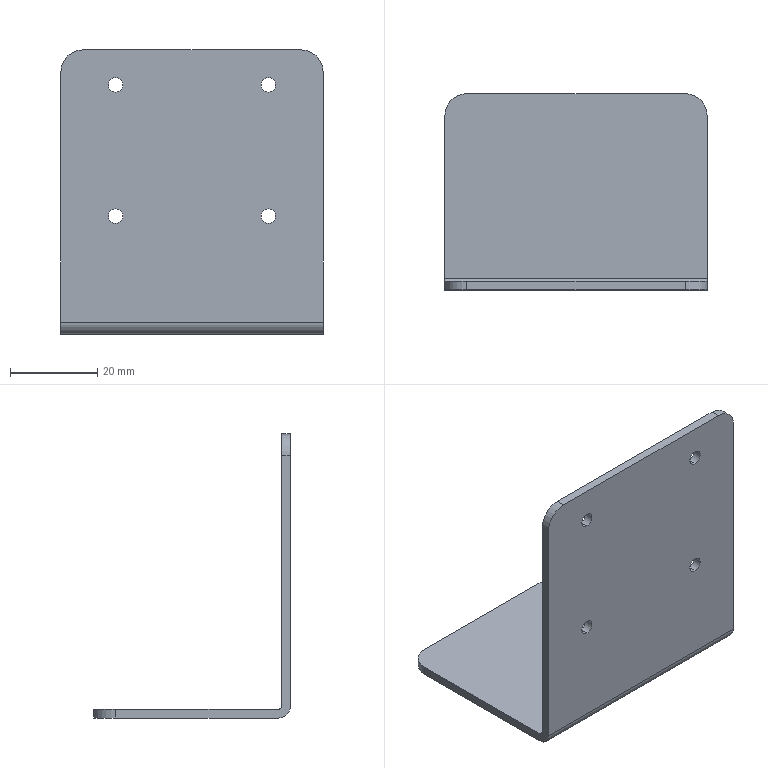Part | 1 solid | 22 faces | box 60 x 45 x 65 mm | volume 12759 mm3 | cylinder 14 | plane 8 | commonest cylinder face diameters 3.3 x8 10 x4 1.48 x1 5.48 x1
STEP:
#1=CARTESIAN_POINT('',(47.5,-2.,-9.65));
#2=VERTEX_POINT('',#1);
#3=CARTESIAN_POINT('',(47.5,-2.,-6.35));
#4=VERTEX_POINT('',#3);
#5=CARTESIAN_POINT('',(47.5,-2.,-8.));
#6=DIRECTION('',(0.,1.,0.));
#7=DIRECTION('',(0.,0.,1.));
#8=AXIS2_PLACEMENT_3D('',#5,#6,#7);
#9=CIRCLE('',#8,1.65);
#10=EDGE_CURVE('',#2,#4,#9,.T.);
#11=ORIENTED_EDGE('',*,*,#10,.F.);
#12=CARTESIAN_POINT('',(47.5,0.,-9.65));
#13=VERTEX_POINT('',#12);
#14=CARTESIAN_POINT('',(47.5,0.,-9.65));
#15=DIRECTION('',(0.,1.,0.));
#16=VECTOR('',#15,1000.);
#17=LINE('',#14,#16);
#18=EDGE_CURVE('',#2,#13,#17,.T.);
#19=ORIENTED_EDGE('',*,*,#18,.T.);
#20=CARTESIAN_POINT('',(47.5,0.,-6.35));
#21=VERTEX_POINT('',#20);
#22=CARTESIAN_POINT('',(47.5,0.,-8.));
#23=DIRECTION('',(0.,1.,0.));
#24=DIRECTION('',(0.,0.,1.));
#25=AXIS2_PLACEMENT_3D('',#22,#23,#24);
#26=CIRCLE('',#25,1.65);
#27=EDGE_CURVE('',#13,#21,#26,.T.);
#28=ORIENTED_EDGE('',*,*,#27,.T.);
#29=CARTESIAN_POINT('',(47.5,0.,-6.35));
#30=DIRECTION('',(0.,1.,0.));
#31=VECTOR('',#30,1000.);
#32=LINE('',#29,#31);
#33=EDGE_CURVE('',#4,#21,#32,.T.);
#34=ORIENTED_EDGE('',*,*,#33,.F.);
#35=EDGE_LOOP('',(#11,#19,#28,#34));
#36=FACE_OUTER_BOUND('',#35,.T.);
#37=CARTESIAN_POINT('',(47.5,0.,-8.));
#38=DIRECTION('',(0.,1.,0.));
#39=DIRECTION('',(0.,0.,1.));
#40=AXIS2_PLACEMENT_3D('',#37,#38,#39);
#41=CYLINDRICAL_SURFACE('',#40,1.65);
#42=ADVANCED_FACE('',(#36),#41,.F.);
#43=CARTESIAN_POINT('',(47.5,-2.,-39.65));
#44=VERTEX_POINT('',#43);
#45=CARTESIAN_POINT('',(47.5,-2.,-36.35));
#46=VERTEX_POINT('',#45);
#47=CARTESIAN_POINT('',(47.5,-2.,-38.));
#48=DIRECTION('',(0.,1.,0.));
#49=DIRECTION('',(0.,0.,1.));
#50=AXIS2_PLACEMENT_3D('',#47,#48,#49);
#51=CIRCLE('',#50,1.65);
#52=EDGE_CURVE('',#44,#46,#51,.T.);
#53=ORIENTED_EDGE('',*,*,#52,.F.);
#54=CARTESIAN_POINT('',(47.5,0.,-39.65));
#55=VERTEX_POINT('',#54);
#56=CARTESIAN_POINT('',(47.5,0.,-39.65));
#57=DIRECTION('',(0.,1.,0.));
#58=VECTOR('',#57,1000.);
#59=LINE('',#56,#58);
#60=EDGE_CURVE('',#44,#55,#59,.T.);
#61=ORIENTED_EDGE('',*,*,#60,.T.);
#62=CARTESIAN_POINT('',(47.5,0.,-36.35));
#63=VERTEX_POINT('',#62);
#64=CARTESIAN_POINT('',(47.5,0.,-38.));
#65=DIRECTION('',(0.,1.,0.));
#66=DIRECTION('',(0.,0.,1.));
#67=AXIS2_PLACEMENT_3D('',#64,#65,#66);
#68=CIRCLE('',#67,1.65);
#69=EDGE_CURVE('',#55,#63,#68,.T.);
#70=ORIENTED_EDGE('',*,*,#69,.T.);
#71=CARTESIAN_POINT('',(47.5,0.,-36.35));
#72=DIRECTION('',(0.,1.,0.));
#73=VECTOR('',#72,1000.);
#74=LINE('',#71,#73);
#75=EDGE_CURVE('',#46,#63,#74,.T.);
#76=ORIENTED_EDGE('',*,*,#75,.F.);
#77=EDGE_LOOP('',(#53,#61,#70,#76));
#78=FACE_OUTER_BOUND('',#77,.T.);
#79=CARTESIAN_POINT('',(47.5,0.,-38.));
#80=DIRECTION('',(0.,1.,0.));
#81=DIRECTION('',(0.,0.,1.));
#82=AXIS2_PLACEMENT_3D('',#79,#80,#81);
#83=CYLINDRICAL_SURFACE('',#82,1.65);
#84=ADVANCED_FACE('',(#78),#83,.F.);
#85=CARTESIAN_POINT('',(12.5,-2.,-9.65));
#86=VERTEX_POINT('',#85);
#87=CARTESIAN_POINT('',(12.5,-2.,-6.35));
#88=VERTEX_POINT('',#87);
#89=CARTESIAN_POINT('',(12.5,-2.,-8.));
#90=DIRECTION('',(0.,1.,0.));
#91=DIRECTION('',(0.,0.,1.));
#92=AXIS2_PLACEMENT_3D('',#89,#90,#91);
#93=CIRCLE('',#92,1.65);
#94=EDGE_CURVE('',#86,#88,#93,.T.);
#95=ORIENTED_EDGE('',*,*,#94,.F.);
#96=CARTESIAN_POINT('',(12.5,0.,-9.65));
#97=VERTEX_POINT('',#96);
#98=CARTESIAN_POINT('',(12.5,0.,-9.65));
#99=DIRECTION('',(0.,1.,0.));
#100=VECTOR('',#99,1000.);
#101=LINE('',#98,#100);
#102=EDGE_CURVE('',#86,#97,#101,.T.);
#103=ORIENTED_EDGE('',*,*,#102,.T.);
#104=CARTESIAN_POINT('',(12.5,0.,-6.35));
#105=VERTEX_POINT('',#104);
#106=CARTESIAN_POINT('',(12.5,0.,-8.));
#107=DIRECTION('',(0.,1.,0.));
#108=DIRECTION('',(0.,0.,1.));
#109=AXIS2_PLACEMENT_3D('',#106,#107,#108);
#110=CIRCLE('',#109,1.65);
#111=EDGE_CURVE('',#97,#105,#110,.T.);
#112=ORIENTED_EDGE('',*,*,#111,.T.);
#113=CARTESIAN_POINT('',(12.5,0.,-6.35));
#114=DIRECTION('',(0.,1.,0.));
#115=VECTOR('',#114,1000.);
#116=LINE('',#113,#115);
#117=EDGE_CURVE('',#88,#105,#116,.T.);
#118=ORIENTED_EDGE('',*,*,#117,.F.);
#119=EDGE_LOOP('',(#95,#103,#112,#118));
#120=FACE_OUTER_BOUND('',#119,.T.);
#121=CARTESIAN_POINT('',(12.5,0.,-8.));
#122=DIRECTION('',(0.,1.,0.));
#123=DIRECTION('',(0.,0.,1.));
#124=AXIS2_PLACEMENT_3D('',#121,#122,#123);
#125=CYLINDRICAL_SURFACE('',#124,1.65);
#126=ADVANCED_FACE('',(#120),#125,.F.);
#127=CARTESIAN_POINT('',(12.5,-2.,-39.65));
#128=VERTEX_POINT('',#127);
#129=CARTESIAN_POINT('',(12.5,-2.,-36.35));
#130=VERTEX_POINT('',#129);
#131=CARTESIAN_POINT('',(12.5,-2.,-38.));
#132=DIRECTION('',(0.,1.,0.));
#133=DIRECTION('',(0.,0.,1.));
#134=AXIS2_PLACEMENT_3D('',#131,#132,#133);
#135=CIRCLE('',#134,1.65);
#136=EDGE_CURVE('',#128,#130,#135,.T.);
#137=ORIENTED_EDGE('',*,*,#136,.F.);
#138=CARTESIAN_POINT('',(12.5,0.,-39.65));
#139=VERTEX_POINT('',#138);
#140=CARTESIAN_POINT('',(12.5,0.,-39.65));
#141=DIRECTION('',(0.,1.,0.));
#142=VECTOR('',#141,1000.);
#143=LINE('',#140,#142);
#144=EDGE_CURVE('',#128,#139,#143,.T.);
#145=ORIENTED_EDGE('',*,*,#144,.T.);
#146=CARTESIAN_POINT('',(12.5,0.,-36.35));
#147=VERTEX_POINT('',#146);
#148=CARTESIAN_POINT('',(12.5,0.,-38.));
#149=DIRECTION('',(0.,1.,0.));
#150=DIRECTION('',(0.,0.,1.));
#151=AXIS2_PLACEMENT_3D('',#148,#149,#150);
#152=CIRCLE('',#151,1.65);
#153=EDGE_CURVE('',#139,#147,#152,.T.);
#154=ORIENTED_EDGE('',*,*,#153,.T.);
#155=CARTESIAN_POINT('',(12.5,0.,-36.35));
#156=DIRECTION('',(0.,1.,0.));
#157=VECTOR('',#156,1000.);
#158=LINE('',#155,#157);
#159=EDGE_CURVE('',#130,#147,#158,.T.);
#160=ORIENTED_EDGE('',*,*,#159,.F.);
#161=EDGE_LOOP('',(#137,#145,#154,#160));
#162=FACE_OUTER_BOUND('',#161,.T.);
#163=CARTESIAN_POINT('',(12.5,0.,-38.));
#164=DIRECTION('',(0.,1.,0.));
#165=DIRECTION('',(0.,0.,1.));
#166=AXIS2_PLACEMENT_3D('',#163,#164,#165);
#167=CYLINDRICAL_SURFACE('',#166,1.65);
#168=ADVANCED_FACE('',(#162),#167,.F.);
#169=CARTESIAN_POINT('',(0.,-2.,-62.26));
#170=VERTEX_POINT('',#169);
#171=CARTESIAN_POINT('',(0.,-2.,-5.));
#172=VERTEX_POINT('',#171);
#173=CARTESIAN_POINT('',(0.,-2.,0.));
#174=DIRECTION('',(0.,0.,1.));
#175=VECTOR('',#174,1000.);
#176=LINE('',#173,#175);
#177=EDGE_CURVE('',#170,#172,#176,.T.);
#178=ORIENTED_EDGE('',*,*,#177,.T.);
#179=CARTESIAN_POINT('',(0.,0.,-5.));
#180=VERTEX_POINT('',#179);
#181=CARTESIAN_POINT('',(0.,-2.,-5.));
#182=DIRECTION('',(0.,1.,0.));
#183=VECTOR('',#182,1000.);
#184=LINE('',#181,#183);
#185=EDGE_CURVE('',#172,#180,#184,.T.);
#186=ORIENTED_EDGE('',*,*,#185,.T.);
#187=CARTESIAN_POINT('',(0.,0.,-62.26));
#188=VERTEX_POINT('',#187);
#189=CARTESIAN_POINT('',(0.,0.,0.));
#190=DIRECTION('',(0.,0.,1.));
#191=VECTOR('',#190,1000.);
#192=LINE('',#189,#191);
#193=EDGE_CURVE('',#188,#180,#192,.T.);
#194=ORIENTED_EDGE('',*,*,#193,.F.);
#195=CARTESIAN_POINT('',(0.,0.74,-63.));
#196=VERTEX_POINT('',#195);
#197=CARTESIAN_POINT('',(0.,0.74,-62.26));
#198=DIRECTION('',(-1.,0.,0.));
#199=DIRECTION('',(0.,0.,1.));
#200=AXIS2_PLACEMENT_3D('',#197,#198,#199);
#201=CIRCLE('',#200,0.74);
#202=EDGE_CURVE('',#196,#188,#201,.T.);
#203=ORIENTED_EDGE('',*,*,#202,.F.);
#204=CARTESIAN_POINT('',(0.,38.,-63.));
#205=VERTEX_POINT('',#204);
#206=CARTESIAN_POINT('',(0.,0.,-63.));
#207=DIRECTION('',(0.,-1.,0.));
#208=VECTOR('',#207,1000.);
#209=LINE('',#206,#208);
#210=EDGE_CURVE('',#205,#196,#209,.T.);
#211=ORIENTED_EDGE('',*,*,#210,.F.);
#212=CARTESIAN_POINT('',(0.,38.,-65.));
#213=VERTEX_POINT('',#212);
#214=CARTESIAN_POINT('',(0.,38.,-65.));
#215=DIRECTION('',(0.,0.,-1.));
#216=VECTOR('',#215,1000.);
#217=LINE('',#214,#216);
#218=EDGE_CURVE('',#205,#213,#217,.T.);
#219=ORIENTED_EDGE('',*,*,#218,.T.);
#220=CARTESIAN_POINT('',(0.,0.74,-65.));
#221=VERTEX_POINT('',#220);
#222=CARTESIAN_POINT('',(0.,0.,-65.));
#223=DIRECTION('',(0.,-1.,0.));
#224=VECTOR('',#223,1000.);
#225=LINE('',#222,#224);
#226=EDGE_CURVE('',#213,#221,#225,.T.);
#227=ORIENTED_EDGE('',*,*,#226,.T.);
#228=CARTESIAN_POINT('',(0.,0.74,-62.26));
#229=DIRECTION('',(-1.,0.,0.));
#230=DIRECTION('',(0.,0.,1.));
#231=AXIS2_PLACEMENT_3D('',#228,#229,#230);
#232=CIRCLE('',#231,2.74);
#233=EDGE_CURVE('',#221,#170,#232,.T.);
#234=ORIENTED_EDGE('',*,*,#233,.T.);
#235=EDGE_LOOP('',(#178,#186,#194,#203,#211,#219,#227,#234));
#236=FACE_OUTER_BOUND('',#235,.T.);
#237=CARTESIAN_POINT('',(0.,-2.,0.));
#238=DIRECTION('',(-1.,0.,0.));
#239=DIRECTION('',(0.,0.,1.));
#240=AXIS2_PLACEMENT_3D('',#237,#238,#239);
#241=PLANE('',#240);
#242=ADVANCED_FACE('',(#236),#241,.T.);
#243=CARTESIAN_POINT('',(47.5,-2.,-8.));
#244=DIRECTION('',(0.,1.,0.));
#245=DIRECTION('',(0.,0.,1.));
#246=AXIS2_PLACEMENT_3D('',#243,#244,#245);
#247=CIRCLE('',#246,1.65);
#248=EDGE_CURVE('',#4,#2,#247,.T.);
#249=ORIENTED_EDGE('',*,*,#248,.T.);
#250=ORIENTED_EDGE('',*,*,#10,.T.);
#251=EDGE_LOOP('',(#249,#250));
#252=FACE_BOUND('',#251,.T.);
#253=CARTESIAN_POINT('',(47.5,-2.,-38.));
#254=DIRECTION('',(0.,1.,0.));
#255=DIRECTION('',(0.,0.,1.));
#256=AXIS2_PLACEMENT_3D('',#253,#254,#255);
#257=CIRCLE('',#256,1.65);
#258=EDGE_CURVE('',#46,#44,#257,.T.);
#259=ORIENTED_EDGE('',*,*,#258,.T.);
#260=ORIENTED_EDGE('',*,*,#52,.T.);
#261=EDGE_LOOP('',(#259,#260));
#262=FACE_BOUND('',#261,.T.);
#263=CARTESIAN_POINT('',(12.5,-2.,-8.));
#264=DIRECTION('',(0.,1.,0.));
#265=DIRECTION('',(0.,0.,1.));
#266=AXIS2_PLACEMENT_3D('',#263,#264,#265);
#267=CIRCLE('',#266,1.65);
#268=EDGE_CURVE('',#88,#86,#267,.T.);
#269=ORIENTED_EDGE('',*,*,#268,.T.);
#270=ORIENTED_EDGE('',*,*,#94,.T.);
#271=EDGE_LOOP('',(#269,#270));
#272=FACE_BOUND('',#271,.T.);
#273=CARTESIAN_POINT('',(12.5,-2.,-38.));
#274=DIRECTION('',(0.,1.,0.));
#275=DIRECTION('',(0.,0.,1.));
#276=AXIS2_PLACEMENT_3D('',#273,#274,#275);
#277=CIRCLE('',#276,1.65);
#278=EDGE_CURVE('',#130,#128,#277,.T.);
#279=ORIENTED_EDGE('',*,*,#278,.T.);
#280=ORIENTED_EDGE('',*,*,#136,.T.);
#281=EDGE_LOOP('',(#279,#280));
#282=FACE_BOUND('',#281,.T.);
#283=CARTESIAN_POINT('',(60.,-2.,-5.));
#284=VERTEX_POINT('',#283);
#285=CARTESIAN_POINT('',(60.,-2.,-62.26));
#286=VERTEX_POINT('',#285);
#287=CARTESIAN_POINT('',(60.,-2.,0.));
#288=DIRECTION('',(0.,0.,-1.));
#289=VECTOR('',#288,1000.);
#290=LINE('',#287,#289);
#291=EDGE_CURVE('',#284,#286,#290,.T.);
#292=ORIENTED_EDGE('',*,*,#291,.F.);
#293=CARTESIAN_POINT('',(55.,-2.,0.));
#294=VERTEX_POINT('',#293);
#295=CARTESIAN_POINT('',(55.,-2.,-5.));
#296=DIRECTION('',(0.,-1.,0.));
#297=DIRECTION('',(0.,0.,-1.));
#298=AXIS2_PLACEMENT_3D('',#295,#296,#297);
#299=CIRCLE('',#298,5.);
#300=EDGE_CURVE('',#284,#294,#299,.T.);
#301=ORIENTED_EDGE('',*,*,#300,.T.);
#302=CARTESIAN_POINT('',(5.,-2.,0.));
#303=VERTEX_POINT('',#302);
#304=CARTESIAN_POINT('',(0.,-2.,0.));
#305=DIRECTION('',(1.,0.,0.));
#306=VECTOR('',#305,1000.);
#307=LINE('',#304,#306);
#308=EDGE_CURVE('',#303,#294,#307,.T.);
#309=ORIENTED_EDGE('',*,*,#308,.F.);
#310=CARTESIAN_POINT('',(5.,-2.,-5.));
#311=DIRECTION('',(0.,-1.,0.));
#312=DIRECTION('',(0.,0.,-1.));
#313=AXIS2_PLACEMENT_3D('',#310,#311,#312);
#314=CIRCLE('',#313,5.);
#315=EDGE_CURVE('',#303,#172,#314,.T.);
#316=ORIENTED_EDGE('',*,*,#315,.T.);
#317=ORIENTED_EDGE('',*,*,#177,.F.);
#318=CARTESIAN_POINT('',(0.,-2.,-62.26));
#319=DIRECTION('',(1.,0.,0.));
#320=VECTOR('',#319,1000.);
#321=LINE('',#318,#320);
#322=EDGE_CURVE('',#170,#286,#321,.T.);
#323=ORIENTED_EDGE('',*,*,#322,.T.);
#324=EDGE_LOOP('',(#292,#301,#309,#316,#317,#323));
#325=FACE_OUTER_BOUND('',#324,.T.);
#326=CARTESIAN_POINT('',(0.,-2.,0.));
#327=DIRECTION('',(0.,-1.,0.));
#328=DIRECTION('',(0.,0.,-1.));
#329=AXIS2_PLACEMENT_3D('',#326,#327,#328);
#330=PLANE('',#329);
#331=ADVANCED_FACE('',(#252,#262,#272,#282,#325),#330,.T.);
#332=CARTESIAN_POINT('',(47.5,0.,-8.));
#333=DIRECTION('',(0.,1.,0.));
#334=DIRECTION('',(0.,0.,1.));
#335=AXIS2_PLACEMENT_3D('',#332,#333,#334);
#336=CIRCLE('',#335,1.65);
#337=EDGE_CURVE('',#21,#13,#336,.T.);
#338=ORIENTED_EDGE('',*,*,#337,.F.);
#339=ORIENTED_EDGE('',*,*,#27,.F.);
#340=EDGE_LOOP('',(#338,#339));
#341=FACE_BOUND('',#340,.T.);
#342=CARTESIAN_POINT('',(47.5,0.,-38.));
#343=DIRECTION('',(0.,1.,0.));
#344=DIRECTION('',(0.,0.,1.));
#345=AXIS2_PLACEMENT_3D('',#342,#343,#344);
#346=CIRCLE('',#345,1.65);
#347=EDGE_CURVE('',#63,#55,#346,.T.);
#348=ORIENTED_EDGE('',*,*,#347,.F.);
#349=ORIENTED_EDGE('',*,*,#69,.F.);
#350=EDGE_LOOP('',(#348,#349));
#351=FACE_BOUND('',#350,.T.);
#352=CARTESIAN_POINT('',(12.5,0.,-8.));
#353=DIRECTION('',(0.,1.,0.));
#354=DIRECTION('',(0.,0.,1.));
#355=AXIS2_PLACEMENT_3D('',#352,#353,#354);
#356=CIRCLE('',#355,1.65);
#357=EDGE_CURVE('',#105,#97,#356,.T.);
#358=ORIENTED_EDGE('',*,*,#357,.F.);
#359=ORIENTED_EDGE('',*,*,#111,.F.);
#360=EDGE_LOOP('',(#358,#359));
#361=FACE_BOUND('',#360,.T.);
#362=CARTESIAN_POINT('',(12.5,0.,-38.));
#363=DIRECTION('',(0.,1.,0.));
#364=DIRECTION('',(0.,0.,1.));
#365=AXIS2_PLACEMENT_3D('',#362,#363,#364);
#366=CIRCLE('',#365,1.65);
#367=EDGE_CURVE('',#147,#139,#366,.T.);
#368=ORIENTED_EDGE('',*,*,#367,.F.);
#369=ORIENTED_EDGE('',*,*,#153,.F.);
#370=EDGE_LOOP('',(#368,#369));
#371=FACE_BOUND('',#370,.T.);
#372=CARTESIAN_POINT('',(5.,0.,0.));
#373=VERTEX_POINT('',#372);
#374=CARTESIAN_POINT('',(55.,0.,0.));
#375=VERTEX_POINT('',#374);
#376=CARTESIAN_POINT('',(0.,0.,0.));
#377=DIRECTION('',(1.,0.,0.));
#378=VECTOR('',#377,1000.);
#379=LINE('',#376,#378);
#380=EDGE_CURVE('',#373,#375,#379,.T.);
#381=ORIENTED_EDGE('',*,*,#380,.T.);
#382=CARTESIAN_POINT('',(60.,0.,-5.));
#383=VERTEX_POINT('',#382);
#384=CARTESIAN_POINT('',(55.,0.,-5.));
#385=DIRECTION('',(0.,1.,0.));
#386=DIRECTION('',(0.,0.,-1.));
#387=AXIS2_PLACEMENT_3D('',#384,#385,#386);
#388=CIRCLE('',#387,5.);
#389=EDGE_CURVE('',#375,#383,#388,.T.);
#390=ORIENTED_EDGE('',*,*,#389,.T.);
#391=CARTESIAN_POINT('',(60.,0.,-62.26));
#392=VERTEX_POINT('',#391);
#393=CARTESIAN_POINT('',(60.,0.,0.));
#394=DIRECTION('',(0.,0.,-1.));
#395=VECTOR('',#394,1000.);
#396=LINE('',#393,#395);
#397=EDGE_CURVE('',#383,#392,#396,.T.);
#398=ORIENTED_EDGE('',*,*,#397,.T.);
#399=CARTESIAN_POINT('',(0.,0.,-62.26));
#400=DIRECTION('',(1.,0.,0.));
#401=VECTOR('',#400,1000.);
#402=LINE('',#399,#401);
#403=EDGE_CURVE('',#188,#392,#402,.T.);
#404=ORIENTED_EDGE('',*,*,#403,.F.);
#405=ORIENTED_EDGE('',*,*,#193,.T.);
#406=CARTESIAN_POINT('',(5.,0.,-5.));
#407=DIRECTION('',(0.,1.,0.));
#408=DIRECTION('',(0.,0.,-1.));
#409=AXIS2_PLACEMENT_3D('',#406,#407,#408);
#410=CIRCLE('',#409,5.);
#411=EDGE_CURVE('',#180,#373,#410,.T.);
#412=ORIENTED_EDGE('',*,*,#411,.T.);
#413=EDGE_LOOP('',(#381,#390,#398,#404,#405,#412));
#414=FACE_OUTER_BOUND('',#413,.T.);
#415=CARTESIAN_POINT('',(0.,0.,0.));
#416=DIRECTION('',(0.,-1.,0.));
#417=DIRECTION('',(0.,0.,-1.));
#418=AXIS2_PLACEMENT_3D('',#415,#416,#417);
#419=PLANE('',#418);
#420=ADVANCED_FACE('',(#341,#351,#361,#371,#414),#419,.F.);
#421=ORIENTED_EDGE('',*,*,#397,.F.);
#422=CARTESIAN_POINT('',(60.,-2.,-5.));
#423=DIRECTION('',(0.,-1.,0.));
#424=VECTOR('',#423,1000.);
#425=LINE('',#422,#424);
#426=EDGE_CURVE('',#383,#284,#425,.T.);
#427=ORIENTED_EDGE('',*,*,#426,.T.);
#428=ORIENTED_EDGE('',*,*,#291,.T.);
#429=CARTESIAN_POINT('',(60.,0.74,-65.));
#430=VERTEX_POINT('',#429);
#431=CARTESIAN_POINT('',(60.,0.74,-62.26));
#432=DIRECTION('',(1.,0.,0.));
#433=DIRECTION('',(0.,0.,1.));
#434=AXIS2_PLACEMENT_3D('',#431,#432,#433);
#435=CIRCLE('',#434,2.74);
#436=EDGE_CURVE('',#286,#430,#435,.T.);
#437=ORIENTED_EDGE('',*,*,#436,.T.);
#438=CARTESIAN_POINT('',(60.,38.,-65.));
#439=VERTEX_POINT('',#438);
#440=CARTESIAN_POINT('',(60.,43.,-65.));
#441=DIRECTION('',(0.,1.,0.));
#442=VECTOR('',#441,1000.);
#443=LINE('',#440,#442);
#444=EDGE_CURVE('',#430,#439,#443,.T.);
#445=ORIENTED_EDGE('',*,*,#444,.T.);
#446=CARTESIAN_POINT('',(60.,38.,-63.));
#447=VERTEX_POINT('',#446);
#448=CARTESIAN_POINT('',(60.,38.,-65.));
#449=DIRECTION('',(0.,0.,1.));
#450=VECTOR('',#449,1000.);
#451=LINE('',#448,#450);
#452=EDGE_CURVE('',#439,#447,#451,.T.);
#453=ORIENTED_EDGE('',*,*,#452,.T.);
#454=CARTESIAN_POINT('',(60.,0.74,-63.));
#455=VERTEX_POINT('',#454);
#456=CARTESIAN_POINT('',(60.,0.,-63.));
#457=DIRECTION('',(0.,1.,0.));
#458=VECTOR('',#457,1000.);
#459=LINE('',#456,#458);
#460=EDGE_CURVE('',#455,#447,#459,.T.);
#461=ORIENTED_EDGE('',*,*,#460,.F.);
#462=CARTESIAN_POINT('',(60.,0.74,-62.26));
#463=DIRECTION('',(1.,0.,0.));
#464=DIRECTION('',(0.,0.,1.));
#465=AXIS2_PLACEMENT_3D('',#462,#463,#464);
#466=CIRCLE('',#465,0.74);
#467=EDGE_CURVE('',#392,#455,#466,.T.);
#468=ORIENTED_EDGE('',*,*,#467,.F.);
#469=EDGE_LOOP('',(#421,#427,#428,#437,#445,#453,#461,#468));
#470=FACE_OUTER_BOUND('',#469,.T.);
#471=CARTESIAN_POINT('',(60.,-2.,0.));
#472=DIRECTION('',(1.,0.,0.));
#473=DIRECTION('',(0.,0.,-1.));
#474=AXIS2_PLACEMENT_3D('',#471,#472,#473);
#475=PLANE('',#474);
#476=ADVANCED_FACE('',(#470),#475,.T.);
#477=ORIENTED_EDGE('',*,*,#308,.T.);
#478=CARTESIAN_POINT('',(55.,-2.,0.));
#479=DIRECTION('',(0.,1.,0.));
#480=VECTOR('',#479,1000.);
#481=LINE('',#478,#480);
#482=EDGE_CURVE('',#294,#375,#481,.T.);
#483=ORIENTED_EDGE('',*,*,#482,.T.);
#484=ORIENTED_EDGE('',*,*,#380,.F.);
#485=CARTESIAN_POINT('',(5.,-2.,0.));
#486=DIRECTION('',(0.,-1.,0.));
#487=VECTOR('',#486,1000.);
#488=LINE('',#485,#487);
#489=EDGE_CURVE('',#373,#303,#488,.T.);
#490=ORIENTED_EDGE('',*,*,#489,.T.);
#491=EDGE_LOOP('',(#477,#483,#484,#490));
#492=FACE_OUTER_BOUND('',#491,.T.);
#493=CARTESIAN_POINT('',(0.,-2.,0.));
#494=DIRECTION('',(0.,0.,1.));
#495=DIRECTION('',(1.,0.,0.));
#496=AXIS2_PLACEMENT_3D('',#493,#494,#495);
#497=PLANE('',#496);
#498=ADVANCED_FACE('',(#492),#497,.T.);
#499=ORIENTED_EDGE('',*,*,#322,.F.);
#500=ORIENTED_EDGE('',*,*,#233,.F.);
#501=CARTESIAN_POINT('',(0.,0.74,-65.));
#502=DIRECTION('',(-1.,0.,0.));
#503=VECTOR('',#502,1000.);
#504=LINE('',#501,#503);
#505=EDGE_CURVE('',#430,#221,#504,.T.);
#506=ORIENTED_EDGE('',*,*,#505,.F.);
#507=ORIENTED_EDGE('',*,*,#436,.F.);
#508=EDGE_LOOP('',(#499,#500,#506,#507));
#509=FACE_OUTER_BOUND('',#508,.T.);
#510=CARTESIAN_POINT('',(0.,0.74,-62.26));
#511=DIRECTION('',(-1.,0.,0.));
#512=DIRECTION('',(0.,0.,-1.));
#513=AXIS2_PLACEMENT_3D('',#510,#511,#512);
#514=CYLINDRICAL_SURFACE('',#513,2.74);
#515=ADVANCED_FACE('',(#509),#514,.T.);
#516=ORIENTED_EDGE('',*,*,#403,.T.);
#517=ORIENTED_EDGE('',*,*,#467,.T.);
#518=CARTESIAN_POINT('',(60.,0.74,-63.));
#519=DIRECTION('',(-1.,0.,0.));
#520=VECTOR('',#519,1000.);
#521=LINE('',#518,#520);
#522=EDGE_CURVE('',#455,#196,#521,.T.);
#523=ORIENTED_EDGE('',*,*,#522,.T.);
#524=ORIENTED_EDGE('',*,*,#202,.T.);
#525=EDGE_LOOP('',(#516,#517,#523,#524));
#526=FACE_OUTER_BOUND('',#525,.T.);
#527=CARTESIAN_POINT('',(0.,0.74,-62.26));
#528=DIRECTION('',(-1.,0.,0.));
#529=DIRECTION('',(0.,0.,-1.));
#530=AXIS2_PLACEMENT_3D('',#527,#528,#529);
#531=CYLINDRICAL_SURFACE('',#530,0.74);
#532=ADVANCED_FACE('',(#526),#531,.F.);
#533=ORIENTED_EDGE('',*,*,#226,.F.);
#534=CARTESIAN_POINT('',(5.,43.,-65.));
#535=VERTEX_POINT('',#534);
#536=CARTESIAN_POINT('',(5.,38.,-65.));
#537=DIRECTION('',(0.,0.,-1.));
#538=DIRECTION('',(-1.,0.,0.));
#539=AXIS2_PLACEMENT_3D('',#536,#537,#538);
#540=CIRCLE('',#539,5.);
#541=EDGE_CURVE('',#213,#535,#540,.T.);
#542=ORIENTED_EDGE('',*,*,#541,.T.);
#543=CARTESIAN_POINT('',(55.,43.,-65.));
#544=VERTEX_POINT('',#543);
#545=CARTESIAN_POINT('',(0.,43.,-65.));
#546=DIRECTION('',(-1.,0.,0.));
#547=VECTOR('',#546,1000.);
#548=LINE('',#545,#547);
#549=EDGE_CURVE('',#544,#535,#548,.T.);
#550=ORIENTED_EDGE('',*,*,#549,.F.);
#551=CARTESIAN_POINT('',(55.,38.,-65.));
#552=DIRECTION('',(0.,0.,-1.));
#553=DIRECTION('',(-1.,0.,0.));
#554=AXIS2_PLACEMENT_3D('',#551,#552,#553);
#555=CIRCLE('',#554,5.);
#556=EDGE_CURVE('',#544,#439,#555,.T.);
#557=ORIENTED_EDGE('',*,*,#556,.T.);
#558=ORIENTED_EDGE('',*,*,#444,.F.);
#559=ORIENTED_EDGE('',*,*,#505,.T.);
#560=EDGE_LOOP('',(#533,#542,#550,#557,#558,#559));
#561=FACE_OUTER_BOUND('',#560,.T.);
#562=CARTESIAN_POINT('',(0.,0.,-65.));
#563=DIRECTION('',(0.,0.,-1.));
#564=DIRECTION('',(-1.,0.,0.));
#565=AXIS2_PLACEMENT_3D('',#562,#563,#564);
#566=PLANE('',#565);
#567=ADVANCED_FACE('',(#561),#566,.T.);
#568=CARTESIAN_POINT('',(55.,43.,-63.));
#569=VERTEX_POINT('',#568);
#570=CARTESIAN_POINT('',(5.,43.,-63.));
#571=VERTEX_POINT('',#570);
#572=CARTESIAN_POINT('',(0.,43.,-63.));
#573=DIRECTION('',(-1.,0.,0.));
#574=VECTOR('',#573,1000.);
#575=LINE('',#572,#574);
#576=EDGE_CURVE('',#569,#571,#575,.T.);
#577=ORIENTED_EDGE('',*,*,#576,.T.);
#578=CARTESIAN_POINT('',(5.,38.,-63.));
#579=DIRECTION('',(0.,0.,1.));
#580=DIRECTION('',(-1.,0.,0.));
#581=AXIS2_PLACEMENT_3D('',#578,#579,#580);
#582=CIRCLE('',#581,5.);
#583=EDGE_CURVE('',#571,#205,#582,.T.);
#584=ORIENTED_EDGE('',*,*,#583,.T.);
#585=ORIENTED_EDGE('',*,*,#210,.T.);
#586=ORIENTED_EDGE('',*,*,#522,.F.);
#587=ORIENTED_EDGE('',*,*,#460,.T.);
#588=CARTESIAN_POINT('',(55.,38.,-63.));
#589=DIRECTION('',(0.,0.,1.));
#590=DIRECTION('',(-1.,0.,0.));
#591=AXIS2_PLACEMENT_3D('',#588,#589,#590);
#592=CIRCLE('',#591,5.);
#593=EDGE_CURVE('',#447,#569,#592,.T.);
#594=ORIENTED_EDGE('',*,*,#593,.T.);
#595=EDGE_LOOP('',(#577,#584,#585,#586,#587,#594));
#596=FACE_OUTER_BOUND('',#595,.T.);
#597=CARTESIAN_POINT('',(0.,0.,-63.));
#598=DIRECTION('',(0.,0.,-1.));
#599=DIRECTION('',(-1.,0.,0.));
#600=AXIS2_PLACEMENT_3D('',#597,#598,#599);
#601=PLANE('',#600);
#602=ADVANCED_FACE('',(#596),#601,.F.);
#603=ORIENTED_EDGE('',*,*,#549,.T.);
#604=CARTESIAN_POINT('',(5.,43.,-65.));
#605=DIRECTION('',(0.,0.,1.));
#606=VECTOR('',#605,1000.);
#607=LINE('',#604,#606);
#608=EDGE_CURVE('',#535,#571,#607,.T.);
#609=ORIENTED_EDGE('',*,*,#608,.T.);
#610=ORIENTED_EDGE('',*,*,#576,.F.);
#611=CARTESIAN_POINT('',(55.,43.,-65.));
#612=DIRECTION('',(0.,0.,-1.));
#613=VECTOR('',#612,1000.);
#614=LINE('',#611,#613);
#615=EDGE_CURVE('',#569,#544,#614,.T.);
#616=ORIENTED_EDGE('',*,*,#615,.T.);
#617=EDGE_LOOP('',(#603,#609,#610,#616));
#618=FACE_OUTER_BOUND('',#617,.T.);
#619=CARTESIAN_POINT('',(0.,43.,-65.));
#620=DIRECTION('',(0.,1.,0.));
#621=DIRECTION('',(0.,0.,1.));
#622=AXIS2_PLACEMENT_3D('',#619,#620,#621);
#623=PLANE('',#622);
#624=ADVANCED_FACE('',(#618),#623,.T.);
#625=ORIENTED_EDGE('',*,*,#541,.F.);
#626=ORIENTED_EDGE('',*,*,#218,.F.);
#627=ORIENTED_EDGE('',*,*,#583,.F.);
#628=ORIENTED_EDGE('',*,*,#608,.F.);
#629=EDGE_LOOP('',(#625,#626,#627,#628));
#630=FACE_OUTER_BOUND('',#629,.T.);
#631=CARTESIAN_POINT('',(5.,38.,-65.));
#632=DIRECTION('',(0.,0.,1.));
#633=DIRECTION('',(1.,0.,0.));
#634=AXIS2_PLACEMENT_3D('',#631,#632,#633);
#635=CYLINDRICAL_SURFACE('',#634,5.);
#636=ADVANCED_FACE('',(#630),#635,.T.);
#637=ORIENTED_EDGE('',*,*,#556,.F.);
#638=ORIENTED_EDGE('',*,*,#615,.F.);
#639=ORIENTED_EDGE('',*,*,#593,.F.);
#640=ORIENTED_EDGE('',*,*,#452,.F.);
#641=EDGE_LOOP('',(#637,#638,#639,#640));
#642=FACE_OUTER_BOUND('',#641,.T.);
#643=CARTESIAN_POINT('',(55.,38.,-65.));
#644=DIRECTION('',(0.,0.,1.));
#645=DIRECTION('',(1.,0.,0.));
#646=AXIS2_PLACEMENT_3D('',#643,#644,#645);
#647=CYLINDRICAL_SURFACE('',#646,5.);
#648=ADVANCED_FACE('',(#642),#647,.T.);
#649=ORIENTED_EDGE('',*,*,#300,.F.);
#650=ORIENTED_EDGE('',*,*,#426,.F.);
#651=ORIENTED_EDGE('',*,*,#389,.F.);
#652=ORIENTED_EDGE('',*,*,#482,.F.);
#653=EDGE_LOOP('',(#649,#650,#651,#652));
#654=FACE_OUTER_BOUND('',#653,.T.);
#655=CARTESIAN_POINT('',(55.,-2.,-5.));
#656=DIRECTION('',(0.,1.,0.));
#657=DIRECTION('',(0.,0.,1.));
#658=AXIS2_PLACEMENT_3D('',#655,#656,#657);
#659=CYLINDRICAL_SURFACE('',#658,5.);
#660=ADVANCED_FACE('',(#654),#659,.T.);
#661=ORIENTED_EDGE('',*,*,#315,.F.);
#662=ORIENTED_EDGE('',*,*,#489,.F.);
#663=ORIENTED_EDGE('',*,*,#411,.F.);
#664=ORIENTED_EDGE('',*,*,#185,.F.);
#665=EDGE_LOOP('',(#661,#662,#663,#664));
#666=FACE_OUTER_BOUND('',#665,.T.);
#667=CARTESIAN_POINT('',(5.,-2.,-5.));
#668=DIRECTION('',(0.,1.,0.));
#669=DIRECTION('',(0.,0.,1.));
#670=AXIS2_PLACEMENT_3D('',#667,#668,#669);
#671=CYLINDRICAL_SURFACE('',#670,5.);
#672=ADVANCED_FACE('',(#666),#671,.T.);
#673=ORIENTED_EDGE('',*,*,#144,.F.);
#674=ORIENTED_EDGE('',*,*,#278,.F.);
#675=ORIENTED_EDGE('',*,*,#159,.T.);
#676=ORIENTED_EDGE('',*,*,#367,.T.);
#677=EDGE_LOOP('',(#673,#674,#675,#676));
#678=FACE_OUTER_BOUND('',#677,.T.);
#679=CARTESIAN_POINT('',(12.5,0.,-38.));
#680=DIRECTION('',(0.,1.,0.));
#681=DIRECTION('',(0.,0.,1.));
#682=AXIS2_PLACEMENT_3D('',#679,#680,#681);
#683=CYLINDRICAL_SURFACE('',#682,1.65);
#684=ADVANCED_FACE('',(#678),#683,.F.);
#685=ORIENTED_EDGE('',*,*,#102,.F.);
#686=ORIENTED_EDGE('',*,*,#268,.F.);
#687=ORIENTED_EDGE('',*,*,#117,.T.);
#688=ORIENTED_EDGE('',*,*,#357,.T.);
#689=EDGE_LOOP('',(#685,#686,#687,#688));
#690=FACE_OUTER_BOUND('',#689,.T.);
#691=CARTESIAN_POINT('',(12.5,0.,-8.));
#692=DIRECTION('',(0.,1.,0.));
#693=DIRECTION('',(0.,0.,1.));
#694=AXIS2_PLACEMENT_3D('',#691,#692,#693);
#695=CYLINDRICAL_SURFACE('',#694,1.65);
#696=ADVANCED_FACE('',(#690),#695,.F.);
#697=ORIENTED_EDGE('',*,*,#60,.F.);
#698=ORIENTED_EDGE('',*,*,#258,.F.);
#699=ORIENTED_EDGE('',*,*,#75,.T.);
#700=ORIENTED_EDGE('',*,*,#347,.T.);
#701=EDGE_LOOP('',(#697,#698,#699,#700));
#702=FACE_OUTER_BOUND('',#701,.T.);
#703=CARTESIAN_POINT('',(47.5,0.,-38.));
#704=DIRECTION('',(0.,1.,0.));
#705=DIRECTION('',(0.,0.,1.));
#706=AXIS2_PLACEMENT_3D('',#703,#704,#705);
#707=CYLINDRICAL_SURFACE('',#706,1.65);
#708=ADVANCED_FACE('',(#702),#707,.F.);
#709=ORIENTED_EDGE('',*,*,#18,.F.);
#710=ORIENTED_EDGE('',*,*,#248,.F.);
#711=ORIENTED_EDGE('',*,*,#33,.T.);
#712=ORIENTED_EDGE('',*,*,#337,.T.);
#713=EDGE_LOOP('',(#709,#710,#711,#712));
#714=FACE_OUTER_BOUND('',#713,.T.);
#715=CARTESIAN_POINT('',(47.5,0.,-8.));
#716=DIRECTION('',(0.,1.,0.));
#717=DIRECTION('',(0.,0.,1.));
#718=AXIS2_PLACEMENT_3D('',#715,#716,#717);
#719=CYLINDRICAL_SURFACE('',#718,1.65);
#720=ADVANCED_FACE('',(#714),#719,.F.);
#721=CLOSED_SHELL('',(#42,#84,#126,#168,#242,#331,#420,#476,#498,#515,#532,#567,#602,#624,#636,#648,#660,#672,#684,#696,#708,#720));
#722=MANIFOLD_SOLID_BREP('',#721);
#723=CARTESIAN_POINT('',(0.,0.,0.));
#724=DIRECTION('',(0.,0.,1.));
#725=DIRECTION('',(1.,0.,0.));
#726=AXIS2_PLACEMENT_3D('',#723,#724,#725);
#727=(LENGTH_UNIT()NAMED_UNIT(*)SI_UNIT(.MILLI.,.METRE.));
#728=UNCERTAINTY_MEASURE_WITH_UNIT(LENGTH_MEASURE(0.00001),#727,'','');
#729=(NAMED_UNIT(*)PLANE_ANGLE_UNIT()SI_UNIT($,.RADIAN.));
#730=(NAMED_UNIT(*)SI_UNIT($,.STERADIAN.)SOLID_ANGLE_UNIT());
#731=(GEOMETRIC_REPRESENTATION_CONTEXT(3)GLOBAL_UNCERTAINTY_ASSIGNED_CONTEXT((#728))GLOBAL_UNIT_ASSIGNED_CONTEXT((#727,#729,#730))REPRESENTATION_CONTEXT('',''));
#732=ADVANCED_BREP_SHAPE_REPRESENTATION('',(#722,#726),#731);